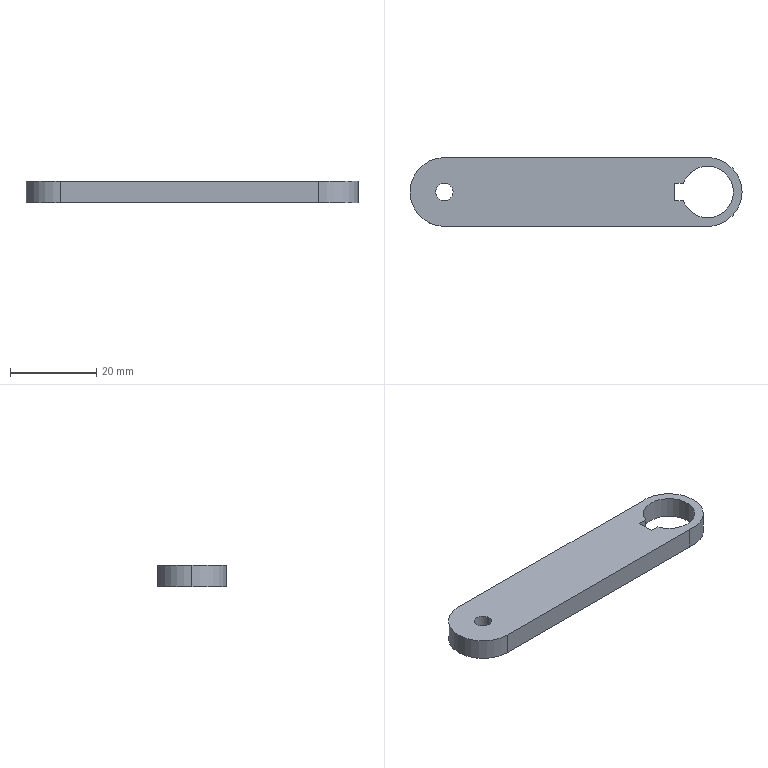Part | SolidWorks | features Extrusion 1 | 1 solid | 13 faces | box 77.185 x 16 x 5 mm | volume 5210 mm3 | plane 7 | cylinder 6 | commonest cylinder face diameters 16 x3 4 x2 12 x1
STEP:
#1=CARTESIAN_POINT('',(-55.731,-0.2687,5.));
#2=VERTEX_POINT('',#1);
#3=CARTESIAN_POINT('',(-51.731,-0.2687,5.));
#4=VERTEX_POINT('',#3);
#5=CARTESIAN_POINT('',(-53.731,-0.2687,5.));
#6=DIRECTION('',(0.,0.,1.));
#7=DIRECTION('',(1.,0.,0.));
#8=AXIS2_PLACEMENT_3D('',#5,#6,#7);
#9=CIRCLE('',#8,2.);
#10=EDGE_CURVE('',#2,#4,#9,.T.);
#11=ORIENTED_EDGE('',*,*,#10,.T.);
#12=CARTESIAN_POINT('',(-51.731,-0.2687,0.));
#13=VERTEX_POINT('',#12);
#14=CARTESIAN_POINT('',(-51.731,-0.2687,5.));
#15=DIRECTION('',(0.,0.,-1.));
#16=VECTOR('',#15,1000.);
#17=LINE('',#14,#16);
#18=EDGE_CURVE('',#4,#13,#17,.T.);
#19=ORIENTED_EDGE('',*,*,#18,.T.);
#20=CARTESIAN_POINT('',(-55.731,-0.2687,0.));
#21=VERTEX_POINT('',#20);
#22=CARTESIAN_POINT('',(-53.731,-0.2687,0.));
#23=DIRECTION('',(0.,0.,1.));
#24=DIRECTION('',(1.,0.,0.));
#25=AXIS2_PLACEMENT_3D('',#22,#23,#24);
#26=CIRCLE('',#25,2.);
#27=EDGE_CURVE('',#21,#13,#26,.T.);
#28=ORIENTED_EDGE('',*,*,#27,.F.);
#29=CARTESIAN_POINT('',(-55.731,-0.2687,5.));
#30=DIRECTION('',(0.,0.,-1.));
#31=VECTOR('',#30,1000.);
#32=LINE('',#29,#31);
#33=EDGE_CURVE('',#2,#21,#32,.T.);
#34=ORIENTED_EDGE('',*,*,#33,.F.);
#35=EDGE_LOOP('',(#11,#19,#28,#34));
#36=FACE_OUTER_BOUND('',#35,.T.);
#37=CARTESIAN_POINT('',(-53.731,-0.2687,5.));
#38=DIRECTION('',(0.,0.,-1.));
#39=DIRECTION('',(-1.,0.,0.));
#40=AXIS2_PLACEMENT_3D('',#37,#38,#39);
#41=CYLINDRICAL_SURFACE('',#40,2.);
#42=ADVANCED_FACE('',(#36),#41,.F.);
#43=CARTESIAN_POINT('',(-61.731,-0.2687,5.));
#44=VERTEX_POINT('',#43);
#45=CARTESIAN_POINT('',(-53.731,-8.269,5.));
#46=VERTEX_POINT('',#45);
#47=CARTESIAN_POINT('',(-53.731,-0.2687,5.));
#48=DIRECTION('',(0.,0.,1.));
#49=DIRECTION('',(1.,0.,0.));
#50=AXIS2_PLACEMENT_3D('',#47,#48,#49);
#51=CIRCLE('',#50,8.);
#52=EDGE_CURVE('',#44,#46,#51,.T.);
#53=ORIENTED_EDGE('',*,*,#52,.F.);
#54=CARTESIAN_POINT('',(-61.731,-0.2687,0.));
#55=VERTEX_POINT('',#54);
#56=CARTESIAN_POINT('',(-61.731,-0.2687,5.));
#57=DIRECTION('',(0.,0.,-1.));
#58=VECTOR('',#57,1000.);
#59=LINE('',#56,#58);
#60=EDGE_CURVE('',#44,#55,#59,.T.);
#61=ORIENTED_EDGE('',*,*,#60,.T.);
#62=CARTESIAN_POINT('',(-53.731,-8.269,0.));
#63=VERTEX_POINT('',#62);
#64=CARTESIAN_POINT('',(-53.731,-0.2687,0.));
#65=DIRECTION('',(0.,0.,1.));
#66=DIRECTION('',(1.,0.,0.));
#67=AXIS2_PLACEMENT_3D('',#64,#65,#66);
#68=CIRCLE('',#67,8.);
#69=EDGE_CURVE('',#55,#63,#68,.T.);
#70=ORIENTED_EDGE('',*,*,#69,.T.);
#71=CARTESIAN_POINT('',(-53.731,-8.269,5.));
#72=DIRECTION('',(0.,0.,-1.));
#73=VECTOR('',#72,1000.);
#74=LINE('',#71,#73);
#75=EDGE_CURVE('',#46,#63,#74,.T.);
#76=ORIENTED_EDGE('',*,*,#75,.F.);
#77=EDGE_LOOP('',(#53,#61,#70,#76));
#78=FACE_OUTER_BOUND('',#77,.T.);
#79=CARTESIAN_POINT('',(-53.731,-0.2687,5.));
#80=DIRECTION('',(0.,0.,-1.));
#81=DIRECTION('',(-1.,0.,0.));
#82=AXIS2_PLACEMENT_3D('',#79,#80,#81);
#83=CYLINDRICAL_SURFACE('',#82,8.);
#84=ADVANCED_FACE('',(#78),#83,.T.);
#85=CARTESIAN_POINT('',(-53.731,7.731,5.));
#86=VERTEX_POINT('',#85);
#87=CARTESIAN_POINT('',(-53.731,-0.2687,5.));
#88=DIRECTION('',(0.,0.,1.));
#89=DIRECTION('',(1.,0.,0.));
#90=AXIS2_PLACEMENT_3D('',#87,#88,#89);
#91=CIRCLE('',#90,8.);
#92=EDGE_CURVE('',#86,#44,#91,.T.);
#93=ORIENTED_EDGE('',*,*,#92,.T.);
#94=ORIENTED_EDGE('',*,*,#52,.T.);
#95=CARTESIAN_POINT('',(6.269,-8.18,5.));
#96=VERTEX_POINT('',#95);
#97=CARTESIAN_POINT('',(-53.731,-8.269,5.));
#98=DIRECTION('',(1.,0.00147,0.));
#99=VECTOR('',#98,1000.);
#100=LINE('',#97,#99);
#101=EDGE_CURVE('',#46,#96,#100,.T.);
#102=ORIENTED_EDGE('',*,*,#101,.T.);
#103=CARTESIAN_POINT('',(6.269,7.643,5.));
#104=VERTEX_POINT('',#103);
#105=CARTESIAN_POINT('',(7.454,-0.2687,5.));
#106=DIRECTION('',(0.,0.,1.));
#107=DIRECTION('',(1.,0.,0.));
#108=AXIS2_PLACEMENT_3D('',#105,#106,#107);
#109=CIRCLE('',#108,8.);
#110=EDGE_CURVE('',#96,#104,#109,.T.);
#111=ORIENTED_EDGE('',*,*,#110,.T.);
#112=CARTESIAN_POINT('',(-53.731,7.731,5.));
#113=DIRECTION('',(-1.,0.00147,0.));
#114=VECTOR('',#113,1000.);
#115=LINE('',#112,#114);
#116=EDGE_CURVE('',#104,#86,#115,.T.);
#117=ORIENTED_EDGE('',*,*,#116,.T.);
#118=EDGE_LOOP('',(#93,#94,#102,#111,#117));
#119=FACE_OUTER_BOUND('',#118,.T.);
#120=ORIENTED_EDGE('',*,*,#10,.F.);
#121=CARTESIAN_POINT('',(-53.731,-0.2687,5.));
#122=DIRECTION('',(0.,0.,1.));
#123=DIRECTION('',(1.,0.,0.));
#124=AXIS2_PLACEMENT_3D('',#121,#122,#123);
#125=CIRCLE('',#124,2.);
#126=EDGE_CURVE('',#4,#2,#125,.T.);
#127=ORIENTED_EDGE('',*,*,#126,.F.);
#128=EDGE_LOOP('',(#120,#127));
#129=FACE_BOUND('',#128,.T.);
#130=CARTESIAN_POINT('',(1.797,1.731,5.));
#131=VERTEX_POINT('',#130);
#132=CARTESIAN_POINT('',(-0.203,1.731,5.));
#133=VERTEX_POINT('',#132);
#134=CARTESIAN_POINT('',(1.797,1.731,5.));
#135=DIRECTION('',(-1.,0.,0.));
#136=VECTOR('',#135,1000.);
#137=LINE('',#134,#136);
#138=EDGE_CURVE('',#131,#133,#137,.T.);
#139=ORIENTED_EDGE('',*,*,#138,.F.);
#140=CARTESIAN_POINT('',(1.797,-2.269,5.));
#141=VERTEX_POINT('',#140);
#142=CARTESIAN_POINT('',(7.454,-0.2687,5.));
#143=DIRECTION('',(0.,0.,1.));
#144=DIRECTION('',(1.,0.,0.));
#145=AXIS2_PLACEMENT_3D('',#142,#143,#144);
#146=CIRCLE('',#145,6.);
#147=EDGE_CURVE('',#141,#131,#146,.T.);
#148=ORIENTED_EDGE('',*,*,#147,.F.);
#149=CARTESIAN_POINT('',(-0.203,-2.269,5.));
#150=VERTEX_POINT('',#149);
#151=CARTESIAN_POINT('',(1.797,-2.269,5.));
#152=DIRECTION('',(1.,0.,0.));
#153=VECTOR('',#152,1000.);
#154=LINE('',#151,#153);
#155=EDGE_CURVE('',#150,#141,#154,.T.);
#156=ORIENTED_EDGE('',*,*,#155,.F.);
#157=CARTESIAN_POINT('',(-0.203,1.731,5.));
#158=DIRECTION('',(0.,-1.,0.));
#159=VECTOR('',#158,1000.);
#160=LINE('',#157,#159);
#161=EDGE_CURVE('',#133,#150,#160,.T.);
#162=ORIENTED_EDGE('',*,*,#161,.F.);
#163=EDGE_LOOP('',(#139,#148,#156,#162));
#164=FACE_BOUND('',#163,.T.);
#165=CARTESIAN_POINT('',(-53.731,-0.2687,5.));
#166=DIRECTION('',(0.,0.,1.));
#167=DIRECTION('',(1.,0.,0.));
#168=AXIS2_PLACEMENT_3D('',#165,#166,#167);
#169=PLANE('',#168);
#170=ADVANCED_FACE('',(#119,#129,#164),#169,.T.);
#171=ORIENTED_EDGE('',*,*,#27,.T.);
#172=CARTESIAN_POINT('',(-53.731,-0.2687,0.));
#173=DIRECTION('',(0.,0.,1.));
#174=DIRECTION('',(1.,0.,0.));
#175=AXIS2_PLACEMENT_3D('',#172,#173,#174);
#176=CIRCLE('',#175,2.);
#177=EDGE_CURVE('',#13,#21,#176,.T.);
#178=ORIENTED_EDGE('',*,*,#177,.T.);
#179=EDGE_LOOP('',(#171,#178));
#180=FACE_BOUND('',#179,.T.);
#181=CARTESIAN_POINT('',(-53.731,7.731,0.));
#182=VERTEX_POINT('',#181);
#183=CARTESIAN_POINT('',(-53.731,-0.2687,0.));
#184=DIRECTION('',(0.,0.,1.));
#185=DIRECTION('',(1.,0.,0.));
#186=AXIS2_PLACEMENT_3D('',#183,#184,#185);
#187=CIRCLE('',#186,8.);
#188=EDGE_CURVE('',#182,#55,#187,.T.);
#189=ORIENTED_EDGE('',*,*,#188,.F.);
#190=CARTESIAN_POINT('',(6.269,7.643,0.));
#191=VERTEX_POINT('',#190);
#192=CARTESIAN_POINT('',(-53.731,7.731,0.));
#193=DIRECTION('',(-1.,0.00147,0.));
#194=VECTOR('',#193,1000.);
#195=LINE('',#192,#194);
#196=EDGE_CURVE('',#191,#182,#195,.T.);
#197=ORIENTED_EDGE('',*,*,#196,.F.);
#198=CARTESIAN_POINT('',(6.269,-8.18,0.));
#199=VERTEX_POINT('',#198);
#200=CARTESIAN_POINT('',(7.454,-0.2687,0.));
#201=DIRECTION('',(0.,0.,1.));
#202=DIRECTION('',(1.,0.,0.));
#203=AXIS2_PLACEMENT_3D('',#200,#201,#202);
#204=CIRCLE('',#203,8.);
#205=EDGE_CURVE('',#199,#191,#204,.T.);
#206=ORIENTED_EDGE('',*,*,#205,.F.);
#207=CARTESIAN_POINT('',(-53.731,-8.269,0.));
#208=DIRECTION('',(1.,0.00147,0.));
#209=VECTOR('',#208,1000.);
#210=LINE('',#207,#209);
#211=EDGE_CURVE('',#63,#199,#210,.T.);
#212=ORIENTED_EDGE('',*,*,#211,.F.);
#213=ORIENTED_EDGE('',*,*,#69,.F.);
#214=EDGE_LOOP('',(#189,#197,#206,#212,#213));
#215=FACE_OUTER_BOUND('',#214,.T.);
#216=CARTESIAN_POINT('',(1.797,-2.269,0.));
#217=VERTEX_POINT('',#216);
#218=CARTESIAN_POINT('',(1.797,1.731,0.));
#219=VERTEX_POINT('',#218);
#220=CARTESIAN_POINT('',(7.454,-0.2687,0.));
#221=DIRECTION('',(0.,0.,1.));
#222=DIRECTION('',(1.,0.,0.));
#223=AXIS2_PLACEMENT_3D('',#220,#221,#222);
#224=CIRCLE('',#223,6.);
#225=EDGE_CURVE('',#217,#219,#224,.T.);
#226=ORIENTED_EDGE('',*,*,#225,.T.);
#227=CARTESIAN_POINT('',(-0.203,1.731,0.));
#228=VERTEX_POINT('',#227);
#229=CARTESIAN_POINT('',(1.797,1.731,0.));
#230=DIRECTION('',(-1.,0.,0.));
#231=VECTOR('',#230,1000.);
#232=LINE('',#229,#231);
#233=EDGE_CURVE('',#219,#228,#232,.T.);
#234=ORIENTED_EDGE('',*,*,#233,.T.);
#235=CARTESIAN_POINT('',(-0.203,-2.269,0.));
#236=VERTEX_POINT('',#235);
#237=CARTESIAN_POINT('',(-0.203,1.731,0.));
#238=DIRECTION('',(0.,-1.,0.));
#239=VECTOR('',#238,1000.);
#240=LINE('',#237,#239);
#241=EDGE_CURVE('',#228,#236,#240,.T.);
#242=ORIENTED_EDGE('',*,*,#241,.T.);
#243=CARTESIAN_POINT('',(1.797,-2.269,0.));
#244=DIRECTION('',(1.,0.,0.));
#245=VECTOR('',#244,1000.);
#246=LINE('',#243,#245);
#247=EDGE_CURVE('',#236,#217,#246,.T.);
#248=ORIENTED_EDGE('',*,*,#247,.T.);
#249=EDGE_LOOP('',(#226,#234,#242,#248));
#250=FACE_BOUND('',#249,.T.);
#251=CARTESIAN_POINT('',(-53.731,-0.2687,0.));
#252=DIRECTION('',(0.,0.,1.));
#253=DIRECTION('',(1.,0.,0.));
#254=AXIS2_PLACEMENT_3D('',#251,#252,#253);
#255=PLANE('',#254);
#256=ADVANCED_FACE('',(#180,#215,#250),#255,.F.);
#257=ORIENTED_EDGE('',*,*,#60,.F.);
#258=ORIENTED_EDGE('',*,*,#92,.F.);
#259=CARTESIAN_POINT('',(-53.731,7.731,5.));
#260=DIRECTION('',(0.,0.,-1.));
#261=VECTOR('',#260,1000.);
#262=LINE('',#259,#261);
#263=EDGE_CURVE('',#86,#182,#262,.T.);
#264=ORIENTED_EDGE('',*,*,#263,.T.);
#265=ORIENTED_EDGE('',*,*,#188,.T.);
#266=EDGE_LOOP('',(#257,#258,#264,#265));
#267=FACE_OUTER_BOUND('',#266,.T.);
#268=CARTESIAN_POINT('',(-53.731,-0.2687,5.));
#269=DIRECTION('',(0.,0.,-1.));
#270=DIRECTION('',(-1.,0.,0.));
#271=AXIS2_PLACEMENT_3D('',#268,#269,#270);
#272=CYLINDRICAL_SURFACE('',#271,8.);
#273=ADVANCED_FACE('',(#267),#272,.T.);
#274=ORIENTED_EDGE('',*,*,#211,.T.);
#275=CARTESIAN_POINT('',(6.269,-8.18,5.));
#276=DIRECTION('',(0.,0.,-1.));
#277=VECTOR('',#276,1000.);
#278=LINE('',#275,#277);
#279=EDGE_CURVE('',#96,#199,#278,.T.);
#280=ORIENTED_EDGE('',*,*,#279,.F.);
#281=ORIENTED_EDGE('',*,*,#101,.F.);
#282=ORIENTED_EDGE('',*,*,#75,.T.);
#283=EDGE_LOOP('',(#274,#280,#281,#282));
#284=FACE_OUTER_BOUND('',#283,.T.);
#285=CARTESIAN_POINT('',(-53.731,-8.269,5.));
#286=DIRECTION('',(-0.00147,1.,0.));
#287=DIRECTION('',(-1.,-0.00147,0.));
#288=AXIS2_PLACEMENT_3D('',#285,#286,#287);
#289=PLANE('',#288);
#290=ADVANCED_FACE('',(#284),#289,.F.);
#291=ORIENTED_EDGE('',*,*,#205,.T.);
#292=CARTESIAN_POINT('',(6.269,7.643,5.));
#293=DIRECTION('',(0.,0.,-1.));
#294=VECTOR('',#293,1000.);
#295=LINE('',#292,#294);
#296=EDGE_CURVE('',#104,#191,#295,.T.);
#297=ORIENTED_EDGE('',*,*,#296,.F.);
#298=ORIENTED_EDGE('',*,*,#110,.F.);
#299=ORIENTED_EDGE('',*,*,#279,.T.);
#300=EDGE_LOOP('',(#291,#297,#298,#299));
#301=FACE_OUTER_BOUND('',#300,.T.);
#302=CARTESIAN_POINT('',(7.454,-0.2687,5.));
#303=DIRECTION('',(0.,0.,-1.));
#304=DIRECTION('',(-1.,0.,0.));
#305=AXIS2_PLACEMENT_3D('',#302,#303,#304);
#306=CYLINDRICAL_SURFACE('',#305,8.);
#307=ADVANCED_FACE('',(#301),#306,.T.);
#308=ORIENTED_EDGE('',*,*,#196,.T.);
#309=ORIENTED_EDGE('',*,*,#263,.F.);
#310=ORIENTED_EDGE('',*,*,#116,.F.);
#311=ORIENTED_EDGE('',*,*,#296,.T.);
#312=EDGE_LOOP('',(#308,#309,#310,#311));
#313=FACE_OUTER_BOUND('',#312,.T.);
#314=CARTESIAN_POINT('',(-53.731,7.731,5.));
#315=DIRECTION('',(-0.00147,-1.,0.));
#316=DIRECTION('',(1.,-0.00147,0.));
#317=AXIS2_PLACEMENT_3D('',#314,#315,#316);
#318=PLANE('',#317);
#319=ADVANCED_FACE('',(#313),#318,.F.);
#320=ORIENTED_EDGE('',*,*,#18,.F.);
#321=ORIENTED_EDGE('',*,*,#126,.T.);
#322=ORIENTED_EDGE('',*,*,#33,.T.);
#323=ORIENTED_EDGE('',*,*,#177,.F.);
#324=EDGE_LOOP('',(#320,#321,#322,#323));
#325=FACE_OUTER_BOUND('',#324,.T.);
#326=CARTESIAN_POINT('',(-53.731,-0.2687,5.));
#327=DIRECTION('',(0.,0.,-1.));
#328=DIRECTION('',(-1.,0.,0.));
#329=AXIS2_PLACEMENT_3D('',#326,#327,#328);
#330=CYLINDRICAL_SURFACE('',#329,2.);
#331=ADVANCED_FACE('',(#325),#330,.F.);
#332=ORIENTED_EDGE('',*,*,#225,.F.);
#333=CARTESIAN_POINT('',(1.797,-2.269,5.));
#334=DIRECTION('',(0.,0.,-1.));
#335=VECTOR('',#334,1000.);
#336=LINE('',#333,#335);
#337=EDGE_CURVE('',#141,#217,#336,.T.);
#338=ORIENTED_EDGE('',*,*,#337,.F.);
#339=ORIENTED_EDGE('',*,*,#147,.T.);
#340=CARTESIAN_POINT('',(1.797,1.731,5.));
#341=DIRECTION('',(0.,0.,-1.));
#342=VECTOR('',#341,1000.);
#343=LINE('',#340,#342);
#344=EDGE_CURVE('',#131,#219,#343,.T.);
#345=ORIENTED_EDGE('',*,*,#344,.T.);
#346=EDGE_LOOP('',(#332,#338,#339,#345));
#347=FACE_OUTER_BOUND('',#346,.T.);
#348=CARTESIAN_POINT('',(7.454,-0.2687,5.));
#349=DIRECTION('',(0.,0.,-1.));
#350=DIRECTION('',(-1.,0.,0.));
#351=AXIS2_PLACEMENT_3D('',#348,#349,#350);
#352=CYLINDRICAL_SURFACE('',#351,6.);
#353=ADVANCED_FACE('',(#347),#352,.F.);
#354=ORIENTED_EDGE('',*,*,#233,.F.);
#355=ORIENTED_EDGE('',*,*,#344,.F.);
#356=ORIENTED_EDGE('',*,*,#138,.T.);
#357=CARTESIAN_POINT('',(-0.203,1.731,5.));
#358=DIRECTION('',(0.,0.,-1.));
#359=VECTOR('',#358,1000.);
#360=LINE('',#357,#359);
#361=EDGE_CURVE('',#133,#228,#360,.T.);
#362=ORIENTED_EDGE('',*,*,#361,.T.);
#363=EDGE_LOOP('',(#354,#355,#356,#362));
#364=FACE_OUTER_BOUND('',#363,.T.);
#365=CARTESIAN_POINT('',(1.797,1.731,5.));
#366=DIRECTION('',(0.,-1.,0.));
#367=DIRECTION('',(1.,0.,0.));
#368=AXIS2_PLACEMENT_3D('',#365,#366,#367);
#369=PLANE('',#368);
#370=ADVANCED_FACE('',(#364),#369,.T.);
#371=ORIENTED_EDGE('',*,*,#241,.F.);
#372=ORIENTED_EDGE('',*,*,#361,.F.);
#373=ORIENTED_EDGE('',*,*,#161,.T.);
#374=CARTESIAN_POINT('',(-0.203,-2.269,5.));
#375=DIRECTION('',(0.,0.,-1.));
#376=VECTOR('',#375,1000.);
#377=LINE('',#374,#376);
#378=EDGE_CURVE('',#150,#236,#377,.T.);
#379=ORIENTED_EDGE('',*,*,#378,.T.);
#380=EDGE_LOOP('',(#371,#372,#373,#379));
#381=FACE_OUTER_BOUND('',#380,.T.);
#382=CARTESIAN_POINT('',(-0.203,1.731,5.));
#383=DIRECTION('',(1.,0.,0.));
#384=DIRECTION('',(0.,1.,0.));
#385=AXIS2_PLACEMENT_3D('',#382,#383,#384);
#386=PLANE('',#385);
#387=ADVANCED_FACE('',(#381),#386,.T.);
#388=ORIENTED_EDGE('',*,*,#247,.F.);
#389=ORIENTED_EDGE('',*,*,#378,.F.);
#390=ORIENTED_EDGE('',*,*,#155,.T.);
#391=ORIENTED_EDGE('',*,*,#337,.T.);
#392=EDGE_LOOP('',(#388,#389,#390,#391));
#393=FACE_OUTER_BOUND('',#392,.T.);
#394=CARTESIAN_POINT('',(1.797,-2.269,5.));
#395=DIRECTION('',(0.,1.,0.));
#396=DIRECTION('',(-1.,0.,0.));
#397=AXIS2_PLACEMENT_3D('',#394,#395,#396);
#398=PLANE('',#397);
#399=ADVANCED_FACE('',(#393),#398,.T.);
#400=CLOSED_SHELL('',(#42,#84,#170,#256,#273,#290,#307,#319,#331,#353,#370,#387,#399));
#401=MANIFOLD_SOLID_BREP('',#400);
#402=CARTESIAN_POINT('',(0.,0.,0.));
#403=DIRECTION('',(0.,0.,1.));
#404=DIRECTION('',(1.,0.,0.));
#405=AXIS2_PLACEMENT_3D('',#402,#403,#404);
#406=(LENGTH_UNIT()NAMED_UNIT(*)SI_UNIT(.MILLI.,.METRE.));
#407=UNCERTAINTY_MEASURE_WITH_UNIT(LENGTH_MEASURE(0.00001),#406,'','');
#408=(NAMED_UNIT(*)PLANE_ANGLE_UNIT()SI_UNIT($,.RADIAN.));
#409=(NAMED_UNIT(*)SI_UNIT($,.STERADIAN.)SOLID_ANGLE_UNIT());
#410=(GEOMETRIC_REPRESENTATION_CONTEXT(3)GLOBAL_UNCERTAINTY_ASSIGNED_CONTEXT((#407))GLOBAL_UNIT_ASSIGNED_CONTEXT((#406,#408,#409))REPRESENTATION_CONTEXT('',''));
#411=ADVANCED_BREP_SHAPE_REPRESENTATION('',(#401,#405),#410);